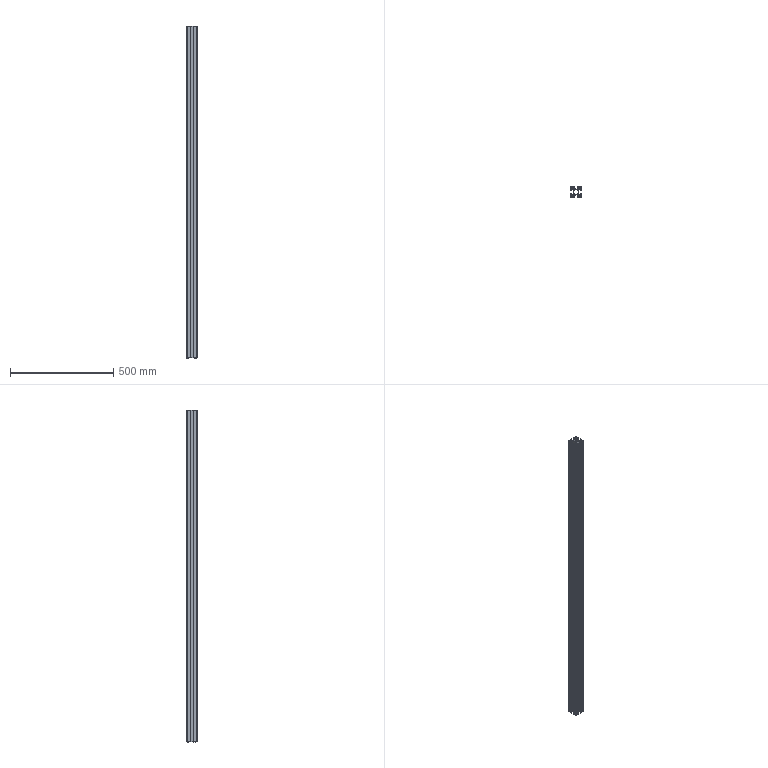Part | STEP file | 46A-00006CC11-1610mm | 1 solid | 142 faces | box 50 x 50 x 1610 mm | volume 945863 mm3 | cylinder 84 | plane 58 | commonest cylinder face diameters 1 x24 4 x24 1.5 x16 3.7 x8 6.7 x8 2 x4